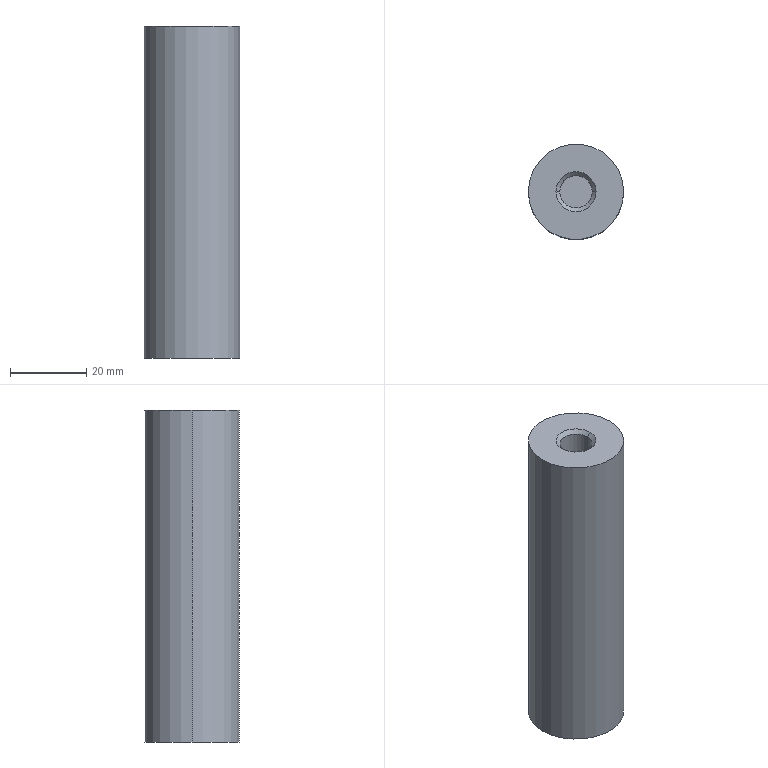Part | SolidWorks | features Chamfer 1, Extrusion 1, Helix 1, ICE 1 | 1 solid | 9 faces | box 25 x 25 x 87 mm | volume 41273 mm3 | cylinder 4 | plane 3 | cone 2 | commonest cylinder face diameters 8.5 x2 25 x2
STEP:
#1=CARTESIAN_POINT('',(-4.25,0.,86.));
#2=VERTEX_POINT('',#1);
#3=CARTESIAN_POINT('',(4.25,0.,86.));
#4=VERTEX_POINT('',#3);
#5=CARTESIAN_POINT('',(0.,0.,86.));
#6=DIRECTION('',(0.,0.,1.));
#7=DIRECTION('',(1.,0.,0.));
#8=AXIS2_PLACEMENT_3D('',#5,#6,#7);
#9=CIRCLE('',#8,4.25);
#10=EDGE_CURVE('',#2,#4,#9,.T.);
#11=ORIENTED_EDGE('',*,*,#10,.F.);
#12=CARTESIAN_POINT('',(-5.25,0.,87.));
#13=VERTEX_POINT('',#12);
#14=CARTESIAN_POINT('',(-4.25,0.,86.));
#15=DIRECTION('',(-0.7071,0.,0.7071));
#16=VECTOR('',#15,1000.);
#17=LINE('',#14,#16);
#18=EDGE_CURVE('',#2,#13,#17,.T.);
#19=ORIENTED_EDGE('',*,*,#18,.T.);
#20=CARTESIAN_POINT('',(5.25,0.,87.));
#21=VERTEX_POINT('',#20);
#22=CARTESIAN_POINT('',(0.,0.,87.));
#23=DIRECTION('',(0.,0.,-1.));
#24=DIRECTION('',(1.,0.,0.));
#25=AXIS2_PLACEMENT_3D('',#22,#23,#24);
#26=CIRCLE('',#25,5.25);
#27=EDGE_CURVE('',#21,#13,#26,.T.);
#28=ORIENTED_EDGE('',*,*,#27,.F.);
#29=CARTESIAN_POINT('',(4.25,0.,86.));
#30=DIRECTION('',(0.7071,0.,0.7071));
#31=VECTOR('',#30,1000.);
#32=LINE('',#29,#31);
#33=EDGE_CURVE('',#4,#21,#32,.T.);
#34=ORIENTED_EDGE('',*,*,#33,.F.);
#35=EDGE_LOOP('',(#11,#19,#28,#34));
#36=FACE_OUTER_BOUND('',#35,.T.);
#37=CARTESIAN_POINT('',(0.,0.,86.));
#38=DIRECTION('',(0.,0.,1.));
#39=DIRECTION('',(1.,0.,0.));
#40=AXIS2_PLACEMENT_3D('',#37,#38,#39);
#41=CONICAL_SURFACE('',#40,4.25,0.7854);
#42=ADVANCED_FACE('',(#36),#41,.F.);
#43=CARTESIAN_POINT('',(-4.25,0.,62.));
#44=VERTEX_POINT('',#43);
#45=CARTESIAN_POINT('',(4.25,0.,62.));
#46=VERTEX_POINT('',#45);
#47=CARTESIAN_POINT('',(0.,0.,62.));
#48=DIRECTION('',(0.,0.,1.));
#49=DIRECTION('',(1.,0.,0.));
#50=AXIS2_PLACEMENT_3D('',#47,#48,#49);
#51=CIRCLE('',#50,4.25);
#52=EDGE_CURVE('',#44,#46,#51,.T.);
#53=ORIENTED_EDGE('',*,*,#52,.F.);
#54=CARTESIAN_POINT('',(-4.25,0.,62.));
#55=DIRECTION('',(0.,0.,1.));
#56=VECTOR('',#55,1000.);
#57=LINE('',#54,#56);
#58=EDGE_CURVE('',#44,#2,#57,.T.);
#59=ORIENTED_EDGE('',*,*,#58,.T.);
#60=ORIENTED_EDGE('',*,*,#10,.T.);
#61=CARTESIAN_POINT('',(4.25,0.,62.));
#62=DIRECTION('',(0.,0.,1.));
#63=VECTOR('',#62,1000.);
#64=LINE('',#61,#63);
#65=EDGE_CURVE('',#46,#4,#64,.T.);
#66=ORIENTED_EDGE('',*,*,#65,.F.);
#67=EDGE_LOOP('',(#53,#59,#60,#66));
#68=FACE_OUTER_BOUND('',#67,.T.);
#69=CARTESIAN_POINT('',(0.,0.,62.));
#70=DIRECTION('',(0.,0.,1.));
#71=DIRECTION('',(1.,0.,0.));
#72=AXIS2_PLACEMENT_3D('',#69,#70,#71);
#73=CYLINDRICAL_SURFACE('',#72,4.25);
#74=ADVANCED_FACE('',(#68),#73,.F.);
#75=CARTESIAN_POINT('',(12.5,0.,87.));
#76=VERTEX_POINT('',#75);
#77=CARTESIAN_POINT('',(-12.5,0.,87.));
#78=VERTEX_POINT('',#77);
#79=CARTESIAN_POINT('',(0.,0.,87.));
#80=DIRECTION('',(0.,0.,1.));
#81=DIRECTION('',(1.,0.,0.));
#82=AXIS2_PLACEMENT_3D('',#79,#80,#81);
#83=CIRCLE('',#82,12.5);
#84=EDGE_CURVE('',#76,#78,#83,.T.);
#85=ORIENTED_EDGE('',*,*,#84,.F.);
#86=CARTESIAN_POINT('',(12.5,0.,0.));
#87=VERTEX_POINT('',#86);
#88=CARTESIAN_POINT('',(12.5,0.,87.));
#89=DIRECTION('',(0.,0.,-1.));
#90=VECTOR('',#89,1000.);
#91=LINE('',#88,#90);
#92=EDGE_CURVE('',#76,#87,#91,.T.);
#93=ORIENTED_EDGE('',*,*,#92,.T.);
#94=CARTESIAN_POINT('',(-12.5,0.,0.));
#95=VERTEX_POINT('',#94);
#96=CARTESIAN_POINT('',(0.,0.,0.));
#97=DIRECTION('',(0.,0.,1.));
#98=DIRECTION('',(1.,0.,0.));
#99=AXIS2_PLACEMENT_3D('',#96,#97,#98);
#100=CIRCLE('',#99,12.5);
#101=EDGE_CURVE('',#87,#95,#100,.T.);
#102=ORIENTED_EDGE('',*,*,#101,.T.);
#103=CARTESIAN_POINT('',(-12.5,0.,87.));
#104=DIRECTION('',(0.,0.,-1.));
#105=VECTOR('',#104,1000.);
#106=LINE('',#103,#105);
#107=EDGE_CURVE('',#78,#95,#106,.T.);
#108=ORIENTED_EDGE('',*,*,#107,.F.);
#109=EDGE_LOOP('',(#85,#93,#102,#108));
#110=FACE_OUTER_BOUND('',#109,.T.);
#111=CARTESIAN_POINT('',(0.,0.,87.));
#112=DIRECTION('',(0.,0.,-1.));
#113=DIRECTION('',(-1.,0.,0.));
#114=AXIS2_PLACEMENT_3D('',#111,#112,#113);
#115=CYLINDRICAL_SURFACE('',#114,12.5);
#116=ADVANCED_FACE('',(#110),#115,.T.);
#117=ORIENTED_EDGE('',*,*,#92,.F.);
#118=CARTESIAN_POINT('',(0.,0.,87.));
#119=DIRECTION('',(0.,0.,1.));
#120=DIRECTION('',(1.,0.,0.));
#121=AXIS2_PLACEMENT_3D('',#118,#119,#120);
#122=CIRCLE('',#121,12.5);
#123=EDGE_CURVE('',#78,#76,#122,.T.);
#124=ORIENTED_EDGE('',*,*,#123,.F.);
#125=ORIENTED_EDGE('',*,*,#107,.T.);
#126=CARTESIAN_POINT('',(0.,0.,0.));
#127=DIRECTION('',(0.,0.,1.));
#128=DIRECTION('',(1.,0.,0.));
#129=AXIS2_PLACEMENT_3D('',#126,#127,#128);
#130=CIRCLE('',#129,12.5);
#131=EDGE_CURVE('',#95,#87,#130,.T.);
#132=ORIENTED_EDGE('',*,*,#131,.T.);
#133=EDGE_LOOP('',(#117,#124,#125,#132));
#134=FACE_OUTER_BOUND('',#133,.T.);
#135=CARTESIAN_POINT('',(0.,0.,87.));
#136=DIRECTION('',(0.,0.,-1.));
#137=DIRECTION('',(-1.,0.,0.));
#138=AXIS2_PLACEMENT_3D('',#135,#136,#137);
#139=CYLINDRICAL_SURFACE('',#138,12.5);
#140=ADVANCED_FACE('',(#134),#139,.T.);
#141=ORIENTED_EDGE('',*,*,#27,.T.);
#142=CARTESIAN_POINT('',(0.,0.,87.));
#143=DIRECTION('',(0.,0.,-1.));
#144=DIRECTION('',(1.,0.,0.));
#145=AXIS2_PLACEMENT_3D('',#142,#143,#144);
#146=CIRCLE('',#145,5.25);
#147=EDGE_CURVE('',#13,#21,#146,.T.);
#148=ORIENTED_EDGE('',*,*,#147,.T.);
#149=EDGE_LOOP('',(#141,#148));
#150=FACE_BOUND('',#149,.T.);
#151=ORIENTED_EDGE('',*,*,#123,.T.);
#152=ORIENTED_EDGE('',*,*,#84,.T.);
#153=EDGE_LOOP('',(#151,#152));
#154=FACE_OUTER_BOUND('',#153,.T.);
#155=CARTESIAN_POINT('',(0.,0.,87.));
#156=DIRECTION('',(0.,0.,1.));
#157=DIRECTION('',(1.,0.,0.));
#158=AXIS2_PLACEMENT_3D('',#155,#156,#157);
#159=PLANE('',#158);
#160=ADVANCED_FACE('',(#150,#154),#159,.T.);
#161=ORIENTED_EDGE('',*,*,#131,.F.);
#162=ORIENTED_EDGE('',*,*,#101,.F.);
#163=EDGE_LOOP('',(#161,#162));
#164=FACE_OUTER_BOUND('',#163,.T.);
#165=CARTESIAN_POINT('',(0.,0.,0.));
#166=DIRECTION('',(0.,0.,1.));
#167=DIRECTION('',(1.,0.,0.));
#168=AXIS2_PLACEMENT_3D('',#165,#166,#167);
#169=PLANE('',#168);
#170=ADVANCED_FACE('',(#164),#169,.F.);
#171=ORIENTED_EDGE('',*,*,#58,.F.);
#172=CARTESIAN_POINT('',(0.,0.,62.));
#173=DIRECTION('',(0.,0.,1.));
#174=DIRECTION('',(1.,0.,0.));
#175=AXIS2_PLACEMENT_3D('',#172,#173,#174);
#176=CIRCLE('',#175,4.25);
#177=EDGE_CURVE('',#46,#44,#176,.T.);
#178=ORIENTED_EDGE('',*,*,#177,.F.);
#179=ORIENTED_EDGE('',*,*,#65,.T.);
#180=CARTESIAN_POINT('',(0.,0.,86.));
#181=DIRECTION('',(0.,0.,1.));
#182=DIRECTION('',(1.,0.,0.));
#183=AXIS2_PLACEMENT_3D('',#180,#181,#182);
#184=CIRCLE('',#183,4.25);
#185=EDGE_CURVE('',#4,#2,#184,.T.);
#186=ORIENTED_EDGE('',*,*,#185,.T.);
#187=EDGE_LOOP('',(#171,#178,#179,#186));
#188=FACE_OUTER_BOUND('',#187,.T.);
#189=CARTESIAN_POINT('',(0.,0.,62.));
#190=DIRECTION('',(0.,0.,1.));
#191=DIRECTION('',(1.,0.,0.));
#192=AXIS2_PLACEMENT_3D('',#189,#190,#191);
#193=CYLINDRICAL_SURFACE('',#192,4.25);
#194=ADVANCED_FACE('',(#188),#193,.F.);
#195=ORIENTED_EDGE('',*,*,#177,.T.);
#196=ORIENTED_EDGE('',*,*,#52,.T.);
#197=EDGE_LOOP('',(#195,#196));
#198=FACE_OUTER_BOUND('',#197,.T.);
#199=CARTESIAN_POINT('',(0.,0.,62.));
#200=DIRECTION('',(0.,0.,1.));
#201=DIRECTION('',(1.,0.,0.));
#202=AXIS2_PLACEMENT_3D('',#199,#200,#201);
#203=PLANE('',#202);
#204=ADVANCED_FACE('',(#198),#203,.T.);
#205=ORIENTED_EDGE('',*,*,#18,.F.);
#206=ORIENTED_EDGE('',*,*,#185,.F.);
#207=ORIENTED_EDGE('',*,*,#33,.T.);
#208=ORIENTED_EDGE('',*,*,#147,.F.);
#209=EDGE_LOOP('',(#205,#206,#207,#208));
#210=FACE_OUTER_BOUND('',#209,.T.);
#211=CARTESIAN_POINT('',(0.,0.,86.));
#212=DIRECTION('',(0.,0.,1.));
#213=DIRECTION('',(1.,0.,0.));
#214=AXIS2_PLACEMENT_3D('',#211,#212,#213);
#215=CONICAL_SURFACE('',#214,4.25,0.7854);
#216=ADVANCED_FACE('',(#210),#215,.F.);
#217=CLOSED_SHELL('',(#42,#74,#116,#140,#160,#170,#194,#204,#216));
#218=MANIFOLD_SOLID_BREP('',#217);
#219=CARTESIAN_POINT('',(0.,0.,0.));
#220=DIRECTION('',(0.,0.,1.));
#221=DIRECTION('',(1.,0.,0.));
#222=AXIS2_PLACEMENT_3D('',#219,#220,#221);
#223=(LENGTH_UNIT()NAMED_UNIT(*)SI_UNIT(.MILLI.,.METRE.));
#224=UNCERTAINTY_MEASURE_WITH_UNIT(LENGTH_MEASURE(0.00001),#223,'','');
#225=(NAMED_UNIT(*)PLANE_ANGLE_UNIT()SI_UNIT($,.RADIAN.));
#226=(NAMED_UNIT(*)SI_UNIT($,.STERADIAN.)SOLID_ANGLE_UNIT());
#227=(GEOMETRIC_REPRESENTATION_CONTEXT(3)GLOBAL_UNCERTAINTY_ASSIGNED_CONTEXT((#224))GLOBAL_UNIT_ASSIGNED_CONTEXT((#223,#225,#226))REPRESENTATION_CONTEXT('',''));
#228=ADVANCED_BREP_SHAPE_REPRESENTATION('',(#218,#222),#227);